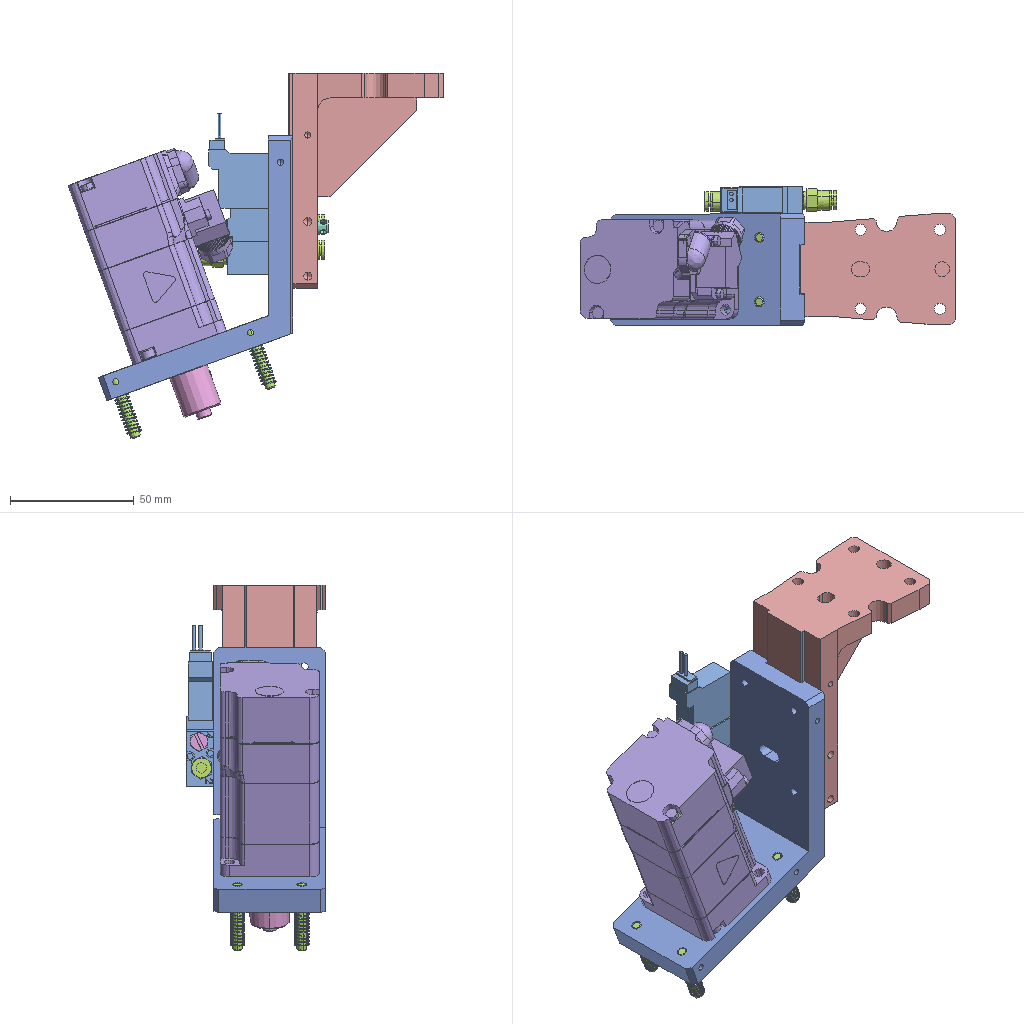Assembly | SolidWorks | 15 different items | 23 placed | box 152 x 56 x 148 mm
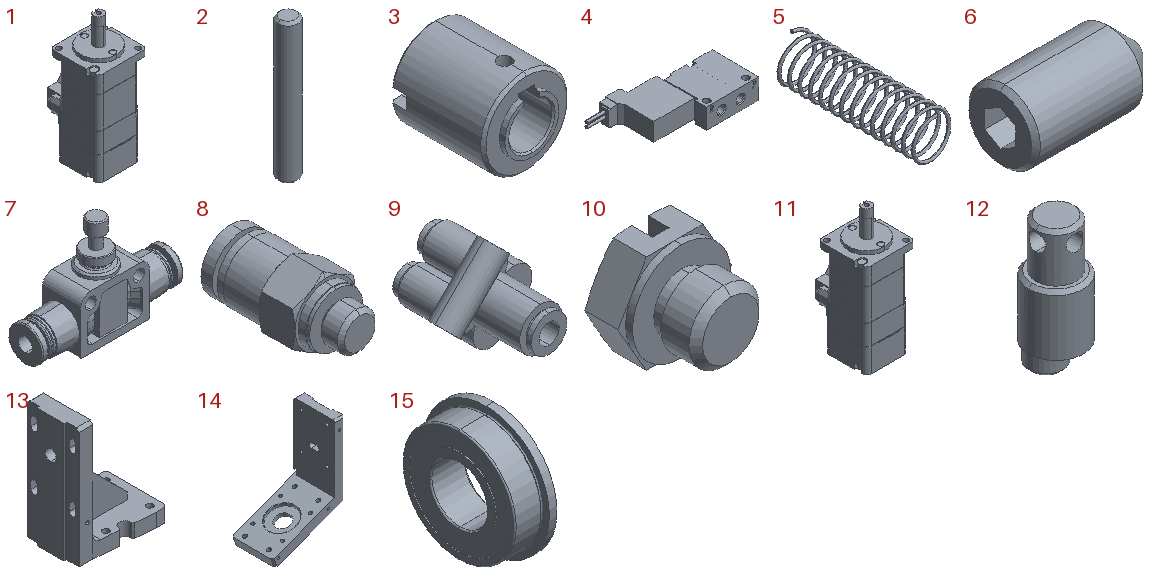Parts list (item | name | quantity | size | volume | features):
1 | (subassembly) | x1 | 41.18 x 54.7 x 102.1 mm | 126795 mm3 | -
2 | - | x4 | 4 x 4 x 28 mm | 346.573 mm3 | features Chamfer 1, Extrusion 1, ICE 1
3 | - | x1 | 16 x 21.1 x 16 mm | 2636 mm3 | features ICE 19, CirPattern 7, Chamfer 3, Extrusion 1, Fillet 1
4 | - | x1 | 65.3 x 33 x 11 mm | 11908 mm3 | features ICE 2, BaseBody 1
5 | - | x4 | 6 x 20.28 x 6 mm | 31.046 mm3 | features Helix 1, RefAxis 1, Sweep 1
6 | - | x1 | 3 x 1.6 x 1.6 mm | 5.006 mm3 | features RevCut 2, Cut 1, LPattern 1, Revolution 1
7 | - | x1 | 40.8 x 11 x 28.611 mm | 4329 mm3 | features BaseBody 1
8 | - | x3 | 8 x 17 x 9.238 mm | 564.577 mm3 | features BaseBody 1
9 | - | x1 | 29.666 x 35.5 x 29.666 mm | 7119 mm3 | features BaseBody 1
10 | - | x1 | 8.083 x 6.5 x 7 mm | 172.442 mm3 | features BaseBody 1
11 | - | x1 | 41.18 x 54.7 x 102.1 mm | 126795 mm3 | features BaseBody 15
12 | - | x1 | 8 x 8 x 19.8 mm | 664.548 mm3 | features ICE 4, Chamfer 1, CirPattern 1, Extrusion 1
13 | - | x1 | 62.8 x 45 x 87 mm | 61473 mm3 | features ICE 10, Chamfer 3, HoleWzd 2, Cut 1, Extrusion 1, Fillet 1, LPattern 1, MirrorPattern 1
14 | - | x1 | 78.596 x 45 x 107.362 mm | 57483 mm3 | features ICE 8, HoleWzd 6, Chamfer 4, 3DProfileFeature 2, MirrorPattern 2, CirPattern 1, Cut 1, Extrusion 1
15 | - | x1 | 5 x 18 x 18 mm | 785.119 mm3 | features RefAxis 3, 3DProfileFeature 1, Revolution 1
Mates (type | each side: item.copy, entity, surface, feature):
Coincident | 14.1 face plane Boss-Extrude1 | 2.1 face plane Boss-Extrude1
Coincident | 14.1 face plane Boss-Extrude1 | 2.2 face plane Boss-Extrude1
Coincident | 14.1 face plane Boss-Extrude1 | 2.3 face plane Boss-Extrude1
Coincident | 14.1 face plane Boss-Extrude1 | 2.4 face plane Boss-Extrude1
Concentric | 14.1 face cylinder Cut-Extrude1 | 15.1 face cylinder Revolve1
DistanceDim | 14.1 face plane Boss-Extrude1 | 15.1 face plane Revolve1
Concentric | 14.1 face cylinder Cut-Extrude3 | 2.2 face cylinder Boss-Extrude1
Concentric | 14.1 face cylinder Cut-Extrude3 | 2.1 face cylinder Boss-Extrude1
Concentric | 14.1 face cylinder Cut-Extrude3 | 2.4 face cylinder Boss-Extrude1
Concentric | 14.1 face cylinder Cut-Extrude3 | 2.3 face cylinder Boss-Extrude1
Concentric | 14.1 edge | 5.1 axis
Concentric | 3.1 face cylinder Cut-Extrude17 | 6.1 face cylinder Base
Coincident | 14.1 face plane Boss-Extrude1 | 13.1 face plane Boss-Extrude1
Width | 13.1 face plane Boss-Extrude1 | 13.1 face plane Boss-Extrude1 | 14.1 face plane Boss-Extrude1 | 14.1 face plane Boss-Extrude1
Parallel | 14.1 face plane Boss-Extrude1 | 2.3 face plane Cut-Extrude1
Coincident | 14.1 face plane Boss-Extrude1 | 4.1 face plane Input1 | 2 times
DistanceDim | 14.1 face plane Boss-Extrude1 | 4.1 face plane Input1
Coincident | 4.1 face plane Input1 | 8.1 face plane Input1
Concentric | 8.1 face cylinder Input1 | 4.1 face cylinder Input1
Coincident | 4.1 face plane Input1 | 10.1 face plane Input1
Concentric | 4.1 face cylinder Input1 | 8.2 face cylinder Input1
Coincident | 4.1 face plane Input1 | 8.2 face plane Input1
DistanceDim | 4.1 face plane Input1 | 14.1 face plane Boss-Extrude1
Concentric | 4.1 face cylinder Input1 | 8.3 face cylinder Input1
Coincident | 4.1 face plane Input1 | 8.3 face plane Input1
Coincident | 13.1 edge | 12.1 face plane Boss-Extrude1
Concentric | 13.1 face cylinder Cut-Extrude8 | 12.1 face cylinder Boss-Extrude2
Tangent | 14.1 face plane Cut-Extrude11 | 12.1 face cylinder Boss-Extrude3
Concentric | 4.1 face cylinder Input1 | 10.1 face cylinder Input1
Coincident | 14.1 face plane Boss-Extrude1 | 11.1 face plane Input1
Concentric | 11.1 face cylinder Input1 | 15.1 face cylinder Revolve1
Parallel | 14.1 face plane Boss-Extrude1 | 11.1 face plane Input1
Concentric | 11.1 face cylinder Input1 | 3.1 face cylinder Cut-Extrude2
Coincident | 3.1 face plane Boss-Extrude5 | 11.1 face plane Input1